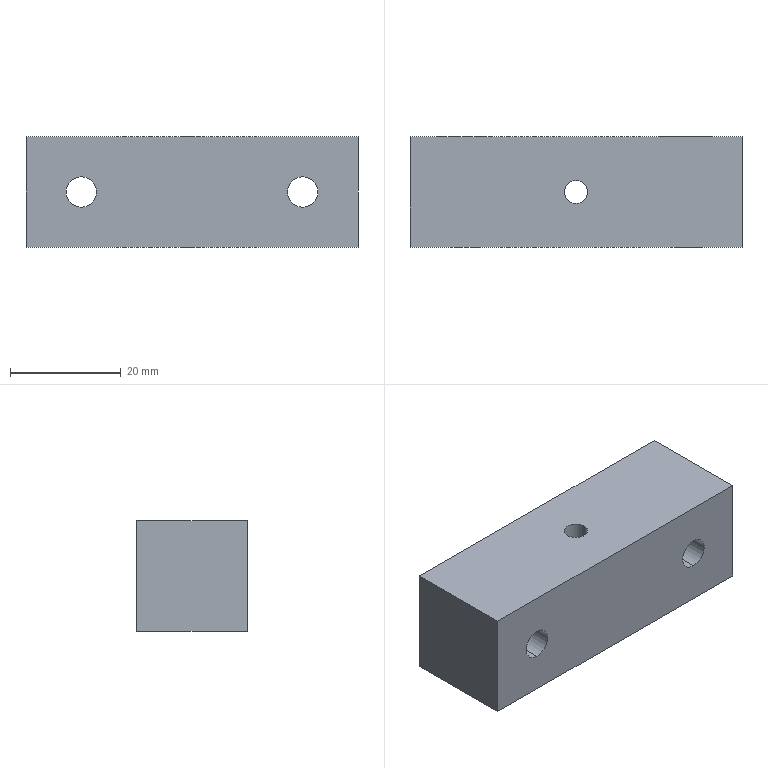Part | SolidWorks | features HoleWzd 2, Extrusion 1 | 1 solid | 18 faces | box 60 x 20 x 20 mm | volume 22148 mm3 | cylinder 10 | plane 8 | commonest cylinder face diameters 5.5 x4 10 x4 4.2 x2
STEP:
#1=CARTESIAN_POINT('',(-2.1,0.,-10.));
#2=VERTEX_POINT('',#1);
#3=CARTESIAN_POINT('',(2.1,0.,-10.));
#4=VERTEX_POINT('',#3);
#5=CARTESIAN_POINT('',(0.,0.,-10.));
#6=DIRECTION('',(0.,0.,1.));
#7=DIRECTION('',(1.,0.,0.));
#8=AXIS2_PLACEMENT_3D('',#5,#6,#7);
#9=CIRCLE('',#8,2.1);
#10=EDGE_CURVE('',#2,#4,#9,.T.);
#11=ORIENTED_EDGE('',*,*,#10,.F.);
#12=CARTESIAN_POINT('',(-2.1,0.,10.));
#13=VERTEX_POINT('',#12);
#14=CARTESIAN_POINT('',(-2.1,0.,10.));
#15=DIRECTION('',(0.,0.,1.));
#16=VECTOR('',#15,1000.);
#17=LINE('',#14,#16);
#18=EDGE_CURVE('',#2,#13,#17,.T.);
#19=ORIENTED_EDGE('',*,*,#18,.T.);
#20=CARTESIAN_POINT('',(2.1,0.,10.));
#21=VERTEX_POINT('',#20);
#22=CARTESIAN_POINT('',(0.,0.,10.));
#23=DIRECTION('',(0.,0.,1.));
#24=DIRECTION('',(1.,0.,0.));
#25=AXIS2_PLACEMENT_3D('',#22,#23,#24);
#26=CIRCLE('',#25,2.1);
#27=EDGE_CURVE('',#13,#21,#26,.T.);
#28=ORIENTED_EDGE('',*,*,#27,.T.);
#29=CARTESIAN_POINT('',(2.1,0.,10.));
#30=DIRECTION('',(0.,0.,1.));
#31=VECTOR('',#30,1000.);
#32=LINE('',#29,#31);
#33=EDGE_CURVE('',#4,#21,#32,.T.);
#34=ORIENTED_EDGE('',*,*,#33,.F.);
#35=EDGE_LOOP('',(#11,#19,#28,#34));
#36=FACE_OUTER_BOUND('',#35,.T.);
#37=CARTESIAN_POINT('',(0.,0.,10.));
#38=DIRECTION('',(0.,0.,1.));
#39=DIRECTION('',(1.,0.,0.));
#40=AXIS2_PLACEMENT_3D('',#37,#38,#39);
#41=CYLINDRICAL_SURFACE('',#40,2.1);
#42=ADVANCED_FACE('',(#36),#41,.F.);
#43=CARTESIAN_POINT('',(20.,4.3,-5.));
#44=VERTEX_POINT('',#43);
#45=CARTESIAN_POINT('',(20.,4.3,5.));
#46=VERTEX_POINT('',#45);
#47=CARTESIAN_POINT('',(20.,4.3,0.));
#48=DIRECTION('',(0.,1.,0.));
#49=DIRECTION('',(0.,0.,1.));
#50=AXIS2_PLACEMENT_3D('',#47,#48,#49);
#51=CIRCLE('',#50,5.);
#52=EDGE_CURVE('',#44,#46,#51,.T.);
#53=ORIENTED_EDGE('',*,*,#52,.F.);
#54=CARTESIAN_POINT('',(20.,10.,-5.));
#55=VERTEX_POINT('',#54);
#56=CARTESIAN_POINT('',(20.,10.,-5.));
#57=DIRECTION('',(0.,1.,0.));
#58=VECTOR('',#57,1000.);
#59=LINE('',#56,#58);
#60=EDGE_CURVE('',#44,#55,#59,.T.);
#61=ORIENTED_EDGE('',*,*,#60,.T.);
#62=CARTESIAN_POINT('',(20.,10.,5.));
#63=VERTEX_POINT('',#62);
#64=CARTESIAN_POINT('',(20.,10.,0.));
#65=DIRECTION('',(0.,1.,0.));
#66=DIRECTION('',(0.,0.,1.));
#67=AXIS2_PLACEMENT_3D('',#64,#65,#66);
#68=CIRCLE('',#67,5.);
#69=EDGE_CURVE('',#55,#63,#68,.T.);
#70=ORIENTED_EDGE('',*,*,#69,.T.);
#71=CARTESIAN_POINT('',(20.,10.,5.));
#72=DIRECTION('',(0.,1.,0.));
#73=VECTOR('',#72,1000.);
#74=LINE('',#71,#73);
#75=EDGE_CURVE('',#46,#63,#74,.T.);
#76=ORIENTED_EDGE('',*,*,#75,.F.);
#77=EDGE_LOOP('',(#53,#61,#70,#76));
#78=FACE_OUTER_BOUND('',#77,.T.);
#79=CARTESIAN_POINT('',(20.,10.,0.));
#80=DIRECTION('',(0.,1.,0.));
#81=DIRECTION('',(0.,0.,1.));
#82=AXIS2_PLACEMENT_3D('',#79,#80,#81);
#83=CYLINDRICAL_SURFACE('',#82,5.);
#84=ADVANCED_FACE('',(#78),#83,.F.);
#85=CARTESIAN_POINT('',(20.,-10.,-2.75));
#86=VERTEX_POINT('',#85);
#87=CARTESIAN_POINT('',(20.,-10.,2.75));
#88=VERTEX_POINT('',#87);
#89=CARTESIAN_POINT('',(20.,-10.,0.));
#90=DIRECTION('',(0.,1.,0.));
#91=DIRECTION('',(0.,0.,1.));
#92=AXIS2_PLACEMENT_3D('',#89,#90,#91);
#93=CIRCLE('',#92,2.75);
#94=EDGE_CURVE('',#86,#88,#93,.T.);
#95=ORIENTED_EDGE('',*,*,#94,.F.);
#96=CARTESIAN_POINT('',(20.,4.3,-2.75));
#97=VERTEX_POINT('',#96);
#98=CARTESIAN_POINT('',(20.,10.,-2.75));
#99=DIRECTION('',(0.,1.,0.));
#100=VECTOR('',#99,1000.);
#101=LINE('',#98,#100);
#102=EDGE_CURVE('',#86,#97,#101,.T.);
#103=ORIENTED_EDGE('',*,*,#102,.T.);
#104=CARTESIAN_POINT('',(20.,4.3,2.75));
#105=VERTEX_POINT('',#104);
#106=CARTESIAN_POINT('',(20.,4.3,0.));
#107=DIRECTION('',(0.,1.,0.));
#108=DIRECTION('',(0.,0.,1.));
#109=AXIS2_PLACEMENT_3D('',#106,#107,#108);
#110=CIRCLE('',#109,2.75);
#111=EDGE_CURVE('',#97,#105,#110,.T.);
#112=ORIENTED_EDGE('',*,*,#111,.T.);
#113=CARTESIAN_POINT('',(20.,10.,2.75));
#114=DIRECTION('',(0.,1.,0.));
#115=VECTOR('',#114,1000.);
#116=LINE('',#113,#115);
#117=EDGE_CURVE('',#88,#105,#116,.T.);
#118=ORIENTED_EDGE('',*,*,#117,.F.);
#119=EDGE_LOOP('',(#95,#103,#112,#118));
#120=FACE_OUTER_BOUND('',#119,.T.);
#121=CARTESIAN_POINT('',(20.,10.,0.));
#122=DIRECTION('',(0.,1.,0.));
#123=DIRECTION('',(0.,0.,1.));
#124=AXIS2_PLACEMENT_3D('',#121,#122,#123);
#125=CYLINDRICAL_SURFACE('',#124,2.75);
#126=ADVANCED_FACE('',(#120),#125,.F.);
#127=CARTESIAN_POINT('',(-20.,4.3,-5.));
#128=VERTEX_POINT('',#127);
#129=CARTESIAN_POINT('',(-20.,4.3,5.));
#130=VERTEX_POINT('',#129);
#131=CARTESIAN_POINT('',(-20.,4.3,0.));
#132=DIRECTION('',(0.,1.,0.));
#133=DIRECTION('',(0.,0.,1.));
#134=AXIS2_PLACEMENT_3D('',#131,#132,#133);
#135=CIRCLE('',#134,5.);
#136=EDGE_CURVE('',#128,#130,#135,.T.);
#137=ORIENTED_EDGE('',*,*,#136,.F.);
#138=CARTESIAN_POINT('',(-20.,10.,-5.));
#139=VERTEX_POINT('',#138);
#140=CARTESIAN_POINT('',(-20.,10.,-5.));
#141=DIRECTION('',(0.,1.,0.));
#142=VECTOR('',#141,1000.);
#143=LINE('',#140,#142);
#144=EDGE_CURVE('',#128,#139,#143,.T.);
#145=ORIENTED_EDGE('',*,*,#144,.T.);
#146=CARTESIAN_POINT('',(-20.,10.,5.));
#147=VERTEX_POINT('',#146);
#148=CARTESIAN_POINT('',(-20.,10.,0.));
#149=DIRECTION('',(0.,1.,0.));
#150=DIRECTION('',(0.,0.,1.));
#151=AXIS2_PLACEMENT_3D('',#148,#149,#150);
#152=CIRCLE('',#151,5.);
#153=EDGE_CURVE('',#139,#147,#152,.T.);
#154=ORIENTED_EDGE('',*,*,#153,.T.);
#155=CARTESIAN_POINT('',(-20.,10.,5.));
#156=DIRECTION('',(0.,1.,0.));
#157=VECTOR('',#156,1000.);
#158=LINE('',#155,#157);
#159=EDGE_CURVE('',#130,#147,#158,.T.);
#160=ORIENTED_EDGE('',*,*,#159,.F.);
#161=EDGE_LOOP('',(#137,#145,#154,#160));
#162=FACE_OUTER_BOUND('',#161,.T.);
#163=CARTESIAN_POINT('',(-20.,10.,0.));
#164=DIRECTION('',(0.,1.,0.));
#165=DIRECTION('',(0.,0.,1.));
#166=AXIS2_PLACEMENT_3D('',#163,#164,#165);
#167=CYLINDRICAL_SURFACE('',#166,5.);
#168=ADVANCED_FACE('',(#162),#167,.F.);
#169=CARTESIAN_POINT('',(-20.,-10.,-2.75));
#170=VERTEX_POINT('',#169);
#171=CARTESIAN_POINT('',(-20.,-10.,2.75));
#172=VERTEX_POINT('',#171);
#173=CARTESIAN_POINT('',(-20.,-10.,0.));
#174=DIRECTION('',(0.,1.,0.));
#175=DIRECTION('',(0.,0.,1.));
#176=AXIS2_PLACEMENT_3D('',#173,#174,#175);
#177=CIRCLE('',#176,2.75);
#178=EDGE_CURVE('',#170,#172,#177,.T.);
#179=ORIENTED_EDGE('',*,*,#178,.F.);
#180=CARTESIAN_POINT('',(-20.,4.3,-2.75));
#181=VERTEX_POINT('',#180);
#182=CARTESIAN_POINT('',(-20.,10.,-2.75));
#183=DIRECTION('',(0.,1.,0.));
#184=VECTOR('',#183,1000.);
#185=LINE('',#182,#184);
#186=EDGE_CURVE('',#170,#181,#185,.T.);
#187=ORIENTED_EDGE('',*,*,#186,.T.);
#188=CARTESIAN_POINT('',(-20.,4.3,2.75));
#189=VERTEX_POINT('',#188);
#190=CARTESIAN_POINT('',(-20.,4.3,0.));
#191=DIRECTION('',(0.,1.,0.));
#192=DIRECTION('',(0.,0.,1.));
#193=AXIS2_PLACEMENT_3D('',#190,#191,#192);
#194=CIRCLE('',#193,2.75);
#195=EDGE_CURVE('',#181,#189,#194,.T.);
#196=ORIENTED_EDGE('',*,*,#195,.T.);
#197=CARTESIAN_POINT('',(-20.,10.,2.75));
#198=DIRECTION('',(0.,1.,0.));
#199=VECTOR('',#198,1000.);
#200=LINE('',#197,#199);
#201=EDGE_CURVE('',#172,#189,#200,.T.);
#202=ORIENTED_EDGE('',*,*,#201,.F.);
#203=EDGE_LOOP('',(#179,#187,#196,#202));
#204=FACE_OUTER_BOUND('',#203,.T.);
#205=CARTESIAN_POINT('',(-20.,10.,0.));
#206=DIRECTION('',(0.,1.,0.));
#207=DIRECTION('',(0.,0.,1.));
#208=AXIS2_PLACEMENT_3D('',#205,#206,#207);
#209=CYLINDRICAL_SURFACE('',#208,2.75);
#210=ADVANCED_FACE('',(#204),#209,.F.);
#211=CARTESIAN_POINT('',(30.,-10.,10.));
#212=VERTEX_POINT('',#211);
#213=CARTESIAN_POINT('',(30.,-10.,-10.));
#214=VERTEX_POINT('',#213);
#215=CARTESIAN_POINT('',(30.,-10.,10.));
#216=DIRECTION('',(0.,0.,-1.));
#217=VECTOR('',#216,1000.);
#218=LINE('',#215,#217);
#219=EDGE_CURVE('',#212,#214,#218,.T.);
#220=ORIENTED_EDGE('',*,*,#219,.T.);
#221=CARTESIAN_POINT('',(30.,10.,-10.));
#222=VERTEX_POINT('',#221);
#223=CARTESIAN_POINT('',(30.,10.,-10.));
#224=DIRECTION('',(0.,-1.,0.));
#225=VECTOR('',#224,1000.);
#226=LINE('',#223,#225);
#227=EDGE_CURVE('',#222,#214,#226,.T.);
#228=ORIENTED_EDGE('',*,*,#227,.F.);
#229=CARTESIAN_POINT('',(30.,10.,10.));
#230=VERTEX_POINT('',#229);
#231=CARTESIAN_POINT('',(30.,10.,10.));
#232=DIRECTION('',(0.,0.,-1.));
#233=VECTOR('',#232,1000.);
#234=LINE('',#231,#233);
#235=EDGE_CURVE('',#230,#222,#234,.T.);
#236=ORIENTED_EDGE('',*,*,#235,.F.);
#237=CARTESIAN_POINT('',(30.,10.,10.));
#238=DIRECTION('',(0.,-1.,0.));
#239=VECTOR('',#238,1000.);
#240=LINE('',#237,#239);
#241=EDGE_CURVE('',#230,#212,#240,.T.);
#242=ORIENTED_EDGE('',*,*,#241,.T.);
#243=EDGE_LOOP('',(#220,#228,#236,#242));
#244=FACE_OUTER_BOUND('',#243,.T.);
#245=CARTESIAN_POINT('',(30.,10.,10.));
#246=DIRECTION('',(-1.,0.,0.));
#247=DIRECTION('',(0.,0.,1.));
#248=AXIS2_PLACEMENT_3D('',#245,#246,#247);
#249=PLANE('',#248);
#250=ADVANCED_FACE('',(#244),#249,.F.);
#251=CARTESIAN_POINT('',(0.,0.,-10.));
#252=DIRECTION('',(0.,0.,1.));
#253=DIRECTION('',(1.,0.,0.));
#254=AXIS2_PLACEMENT_3D('',#251,#252,#253);
#255=CIRCLE('',#254,2.1);
#256=EDGE_CURVE('',#4,#2,#255,.T.);
#257=ORIENTED_EDGE('',*,*,#256,.T.);
#258=ORIENTED_EDGE('',*,*,#10,.T.);
#259=EDGE_LOOP('',(#257,#258));
#260=FACE_BOUND('',#259,.T.);
#261=CARTESIAN_POINT('',(-30.,-10.,-10.));
#262=VERTEX_POINT('',#261);
#263=CARTESIAN_POINT('',(-30.,-10.,-10.));
#264=DIRECTION('',(-1.,0.,0.));
#265=VECTOR('',#264,1000.);
#266=LINE('',#263,#265);
#267=EDGE_CURVE('',#214,#262,#266,.T.);
#268=ORIENTED_EDGE('',*,*,#267,.T.);
#269=CARTESIAN_POINT('',(-30.,10.,-10.));
#270=VERTEX_POINT('',#269);
#271=CARTESIAN_POINT('',(-30.,10.,-10.));
#272=DIRECTION('',(0.,-1.,0.));
#273=VECTOR('',#272,1000.);
#274=LINE('',#271,#273);
#275=EDGE_CURVE('',#270,#262,#274,.T.);
#276=ORIENTED_EDGE('',*,*,#275,.F.);
#277=CARTESIAN_POINT('',(-30.,10.,-10.));
#278=DIRECTION('',(-1.,0.,0.));
#279=VECTOR('',#278,1000.);
#280=LINE('',#277,#279);
#281=EDGE_CURVE('',#222,#270,#280,.T.);
#282=ORIENTED_EDGE('',*,*,#281,.F.);
#283=ORIENTED_EDGE('',*,*,#227,.T.);
#284=EDGE_LOOP('',(#268,#276,#282,#283));
#285=FACE_OUTER_BOUND('',#284,.T.);
#286=CARTESIAN_POINT('',(-30.,10.,-10.));
#287=DIRECTION('',(0.,0.,1.));
#288=DIRECTION('',(1.,0.,0.));
#289=AXIS2_PLACEMENT_3D('',#286,#287,#288);
#290=PLANE('',#289);
#291=ADVANCED_FACE('',(#260,#285),#290,.F.);
#292=CARTESIAN_POINT('',(-30.,-10.,10.));
#293=VERTEX_POINT('',#292);
#294=CARTESIAN_POINT('',(-30.,-10.,10.));
#295=DIRECTION('',(0.,0.,1.));
#296=VECTOR('',#295,1000.);
#297=LINE('',#294,#296);
#298=EDGE_CURVE('',#262,#293,#297,.T.);
#299=ORIENTED_EDGE('',*,*,#298,.T.);
#300=CARTESIAN_POINT('',(-30.,10.,10.));
#301=VERTEX_POINT('',#300);
#302=CARTESIAN_POINT('',(-30.,10.,10.));
#303=DIRECTION('',(0.,-1.,0.));
#304=VECTOR('',#303,1000.);
#305=LINE('',#302,#304);
#306=EDGE_CURVE('',#301,#293,#305,.T.);
#307=ORIENTED_EDGE('',*,*,#306,.F.);
#308=CARTESIAN_POINT('',(-30.,10.,10.));
#309=DIRECTION('',(0.,0.,1.));
#310=VECTOR('',#309,1000.);
#311=LINE('',#308,#310);
#312=EDGE_CURVE('',#270,#301,#311,.T.);
#313=ORIENTED_EDGE('',*,*,#312,.F.);
#314=ORIENTED_EDGE('',*,*,#275,.T.);
#315=EDGE_LOOP('',(#299,#307,#313,#314));
#316=FACE_OUTER_BOUND('',#315,.T.);
#317=CARTESIAN_POINT('',(-30.,10.,10.));
#318=DIRECTION('',(1.,0.,0.));
#319=DIRECTION('',(0.,0.,-1.));
#320=AXIS2_PLACEMENT_3D('',#317,#318,#319);
#321=PLANE('',#320);
#322=ADVANCED_FACE('',(#316),#321,.F.);
#323=CARTESIAN_POINT('',(0.,0.,10.));
#324=DIRECTION('',(0.,0.,1.));
#325=DIRECTION('',(1.,0.,0.));
#326=AXIS2_PLACEMENT_3D('',#323,#324,#325);
#327=CIRCLE('',#326,2.1);
#328=EDGE_CURVE('',#21,#13,#327,.T.);
#329=ORIENTED_EDGE('',*,*,#328,.F.);
#330=ORIENTED_EDGE('',*,*,#27,.F.);
#331=EDGE_LOOP('',(#329,#330));
#332=FACE_BOUND('',#331,.T.);
#333=CARTESIAN_POINT('',(-30.,-10.,10.));
#334=DIRECTION('',(1.,0.,0.));
#335=VECTOR('',#334,1000.);
#336=LINE('',#333,#335);
#337=EDGE_CURVE('',#293,#212,#336,.T.);
#338=ORIENTED_EDGE('',*,*,#337,.T.);
#339=ORIENTED_EDGE('',*,*,#241,.F.);
#340=CARTESIAN_POINT('',(-30.,10.,10.));
#341=DIRECTION('',(1.,0.,0.));
#342=VECTOR('',#341,1000.);
#343=LINE('',#340,#342);
#344=EDGE_CURVE('',#301,#230,#343,.T.);
#345=ORIENTED_EDGE('',*,*,#344,.F.);
#346=ORIENTED_EDGE('',*,*,#306,.T.);
#347=EDGE_LOOP('',(#338,#339,#345,#346));
#348=FACE_OUTER_BOUND('',#347,.T.);
#349=CARTESIAN_POINT('',(-30.,10.,10.));
#350=DIRECTION('',(0.,0.,-1.));
#351=DIRECTION('',(-1.,0.,0.));
#352=AXIS2_PLACEMENT_3D('',#349,#350,#351);
#353=PLANE('',#352);
#354=ADVANCED_FACE('',(#332,#348),#353,.F.);
#355=CARTESIAN_POINT('',(20.,10.,0.));
#356=DIRECTION('',(0.,1.,0.));
#357=DIRECTION('',(0.,0.,1.));
#358=AXIS2_PLACEMENT_3D('',#355,#356,#357);
#359=CIRCLE('',#358,5.);
#360=EDGE_CURVE('',#63,#55,#359,.T.);
#361=ORIENTED_EDGE('',*,*,#360,.F.);
#362=ORIENTED_EDGE('',*,*,#69,.F.);
#363=EDGE_LOOP('',(#361,#362));
#364=FACE_BOUND('',#363,.T.);
#365=CARTESIAN_POINT('',(-20.,10.,0.));
#366=DIRECTION('',(0.,1.,0.));
#367=DIRECTION('',(0.,0.,1.));
#368=AXIS2_PLACEMENT_3D('',#365,#366,#367);
#369=CIRCLE('',#368,5.);
#370=EDGE_CURVE('',#147,#139,#369,.T.);
#371=ORIENTED_EDGE('',*,*,#370,.F.);
#372=ORIENTED_EDGE('',*,*,#153,.F.);
#373=EDGE_LOOP('',(#371,#372));
#374=FACE_BOUND('',#373,.T.);
#375=ORIENTED_EDGE('',*,*,#235,.T.);
#376=ORIENTED_EDGE('',*,*,#281,.T.);
#377=ORIENTED_EDGE('',*,*,#312,.T.);
#378=ORIENTED_EDGE('',*,*,#344,.T.);
#379=EDGE_LOOP('',(#375,#376,#377,#378));
#380=FACE_OUTER_BOUND('',#379,.T.);
#381=CARTESIAN_POINT('',(0.,10.,0.));
#382=DIRECTION('',(0.,-1.,0.));
#383=DIRECTION('',(0.,0.,-1.));
#384=AXIS2_PLACEMENT_3D('',#381,#382,#383);
#385=PLANE('',#384);
#386=ADVANCED_FACE('',(#364,#374,#380),#385,.F.);
#387=CARTESIAN_POINT('',(20.,-10.,0.));
#388=DIRECTION('',(0.,1.,0.));
#389=DIRECTION('',(0.,0.,1.));
#390=AXIS2_PLACEMENT_3D('',#387,#388,#389);
#391=CIRCLE('',#390,2.75);
#392=EDGE_CURVE('',#88,#86,#391,.T.);
#393=ORIENTED_EDGE('',*,*,#392,.T.);
#394=ORIENTED_EDGE('',*,*,#94,.T.);
#395=EDGE_LOOP('',(#393,#394));
#396=FACE_BOUND('',#395,.T.);
#397=CARTESIAN_POINT('',(-20.,-10.,0.));
#398=DIRECTION('',(0.,1.,0.));
#399=DIRECTION('',(0.,0.,1.));
#400=AXIS2_PLACEMENT_3D('',#397,#398,#399);
#401=CIRCLE('',#400,2.75);
#402=EDGE_CURVE('',#172,#170,#401,.T.);
#403=ORIENTED_EDGE('',*,*,#402,.T.);
#404=ORIENTED_EDGE('',*,*,#178,.T.);
#405=EDGE_LOOP('',(#403,#404));
#406=FACE_BOUND('',#405,.T.);
#407=ORIENTED_EDGE('',*,*,#219,.F.);
#408=ORIENTED_EDGE('',*,*,#337,.F.);
#409=ORIENTED_EDGE('',*,*,#298,.F.);
#410=ORIENTED_EDGE('',*,*,#267,.F.);
#411=EDGE_LOOP('',(#407,#408,#409,#410));
#412=FACE_OUTER_BOUND('',#411,.T.);
#413=CARTESIAN_POINT('',(0.,-10.,0.));
#414=DIRECTION('',(0.,-1.,0.));
#415=DIRECTION('',(0.,0.,-1.));
#416=AXIS2_PLACEMENT_3D('',#413,#414,#415);
#417=PLANE('',#416);
#418=ADVANCED_FACE('',(#396,#406,#412),#417,.T.);
#419=ORIENTED_EDGE('',*,*,#186,.F.);
#420=ORIENTED_EDGE('',*,*,#402,.F.);
#421=ORIENTED_EDGE('',*,*,#201,.T.);
#422=CARTESIAN_POINT('',(-20.,4.3,0.));
#423=DIRECTION('',(0.,1.,0.));
#424=DIRECTION('',(0.,0.,1.));
#425=AXIS2_PLACEMENT_3D('',#422,#423,#424);
#426=CIRCLE('',#425,2.75);
#427=EDGE_CURVE('',#189,#181,#426,.T.);
#428=ORIENTED_EDGE('',*,*,#427,.T.);
#429=EDGE_LOOP('',(#419,#420,#421,#428));
#430=FACE_OUTER_BOUND('',#429,.T.);
#431=CARTESIAN_POINT('',(-20.,10.,0.));
#432=DIRECTION('',(0.,1.,0.));
#433=DIRECTION('',(0.,0.,1.));
#434=AXIS2_PLACEMENT_3D('',#431,#432,#433);
#435=CYLINDRICAL_SURFACE('',#434,2.75);
#436=ADVANCED_FACE('',(#430),#435,.F.);
#437=ORIENTED_EDGE('',*,*,#427,.F.);
#438=ORIENTED_EDGE('',*,*,#195,.F.);
#439=EDGE_LOOP('',(#437,#438));
#440=FACE_BOUND('',#439,.T.);
#441=CARTESIAN_POINT('',(-20.,4.3,0.));
#442=DIRECTION('',(0.,1.,0.));
#443=DIRECTION('',(0.,0.,1.));
#444=AXIS2_PLACEMENT_3D('',#441,#442,#443);
#445=CIRCLE('',#444,5.);
#446=EDGE_CURVE('',#130,#128,#445,.T.);
#447=ORIENTED_EDGE('',*,*,#446,.T.);
#448=ORIENTED_EDGE('',*,*,#136,.T.);
#449=EDGE_LOOP('',(#447,#448));
#450=FACE_OUTER_BOUND('',#449,.T.);
#451=CARTESIAN_POINT('',(-17.25,4.3,0.));
#452=DIRECTION('',(0.,-1.,0.));
#453=DIRECTION('',(0.,0.,-1.));
#454=AXIS2_PLACEMENT_3D('',#451,#452,#453);
#455=PLANE('',#454);
#456=ADVANCED_FACE('',(#440,#450),#455,.F.);
#457=ORIENTED_EDGE('',*,*,#144,.F.);
#458=ORIENTED_EDGE('',*,*,#446,.F.);
#459=ORIENTED_EDGE('',*,*,#159,.T.);
#460=ORIENTED_EDGE('',*,*,#370,.T.);
#461=EDGE_LOOP('',(#457,#458,#459,#460));
#462=FACE_OUTER_BOUND('',#461,.T.);
#463=CARTESIAN_POINT('',(-20.,10.,0.));
#464=DIRECTION('',(0.,1.,0.));
#465=DIRECTION('',(0.,0.,1.));
#466=AXIS2_PLACEMENT_3D('',#463,#464,#465);
#467=CYLINDRICAL_SURFACE('',#466,5.);
#468=ADVANCED_FACE('',(#462),#467,.F.);
#469=ORIENTED_EDGE('',*,*,#102,.F.);
#470=ORIENTED_EDGE('',*,*,#392,.F.);
#471=ORIENTED_EDGE('',*,*,#117,.T.);
#472=CARTESIAN_POINT('',(20.,4.3,0.));
#473=DIRECTION('',(0.,1.,0.));
#474=DIRECTION('',(0.,0.,1.));
#475=AXIS2_PLACEMENT_3D('',#472,#473,#474);
#476=CIRCLE('',#475,2.75);
#477=EDGE_CURVE('',#105,#97,#476,.T.);
#478=ORIENTED_EDGE('',*,*,#477,.T.);
#479=EDGE_LOOP('',(#469,#470,#471,#478));
#480=FACE_OUTER_BOUND('',#479,.T.);
#481=CARTESIAN_POINT('',(20.,10.,0.));
#482=DIRECTION('',(0.,1.,0.));
#483=DIRECTION('',(0.,0.,1.));
#484=AXIS2_PLACEMENT_3D('',#481,#482,#483);
#485=CYLINDRICAL_SURFACE('',#484,2.75);
#486=ADVANCED_FACE('',(#480),#485,.F.);
#487=ORIENTED_EDGE('',*,*,#477,.F.);
#488=ORIENTED_EDGE('',*,*,#111,.F.);
#489=EDGE_LOOP('',(#487,#488));
#490=FACE_BOUND('',#489,.T.);
#491=CARTESIAN_POINT('',(20.,4.3,0.));
#492=DIRECTION('',(0.,1.,0.));
#493=DIRECTION('',(0.,0.,1.));
#494=AXIS2_PLACEMENT_3D('',#491,#492,#493);
#495=CIRCLE('',#494,5.);
#496=EDGE_CURVE('',#46,#44,#495,.T.);
#497=ORIENTED_EDGE('',*,*,#496,.T.);
#498=ORIENTED_EDGE('',*,*,#52,.T.);
#499=EDGE_LOOP('',(#497,#498));
#500=FACE_OUTER_BOUND('',#499,.T.);
#501=CARTESIAN_POINT('',(22.75,4.3,0.));
#502=DIRECTION('',(0.,-1.,0.));
#503=DIRECTION('',(0.,0.,-1.));
#504=AXIS2_PLACEMENT_3D('',#501,#502,#503);
#505=PLANE('',#504);
#506=ADVANCED_FACE('',(#490,#500),#505,.F.);
#507=ORIENTED_EDGE('',*,*,#60,.F.);
#508=ORIENTED_EDGE('',*,*,#496,.F.);
#509=ORIENTED_EDGE('',*,*,#75,.T.);
#510=ORIENTED_EDGE('',*,*,#360,.T.);
#511=EDGE_LOOP('',(#507,#508,#509,#510));
#512=FACE_OUTER_BOUND('',#511,.T.);
#513=CARTESIAN_POINT('',(20.,10.,0.));
#514=DIRECTION('',(0.,1.,0.));
#515=DIRECTION('',(0.,0.,1.));
#516=AXIS2_PLACEMENT_3D('',#513,#514,#515);
#517=CYLINDRICAL_SURFACE('',#516,5.);
#518=ADVANCED_FACE('',(#512),#517,.F.);
#519=ORIENTED_EDGE('',*,*,#18,.F.);
#520=ORIENTED_EDGE('',*,*,#256,.F.);
#521=ORIENTED_EDGE('',*,*,#33,.T.);
#522=ORIENTED_EDGE('',*,*,#328,.T.);
#523=EDGE_LOOP('',(#519,#520,#521,#522));
#524=FACE_OUTER_BOUND('',#523,.T.);
#525=CARTESIAN_POINT('',(0.,0.,10.));
#526=DIRECTION('',(0.,0.,1.));
#527=DIRECTION('',(1.,0.,0.));
#528=AXIS2_PLACEMENT_3D('',#525,#526,#527);
#529=CYLINDRICAL_SURFACE('',#528,2.1);
#530=ADVANCED_FACE('',(#524),#529,.F.);
#531=CLOSED_SHELL('',(#42,#84,#126,#168,#210,#250,#291,#322,#354,#386,#418,#436,#456,#468,#486,#506,#518,#530));
#532=MANIFOLD_SOLID_BREP('',#531);
#533=CARTESIAN_POINT('',(0.,0.,0.));
#534=DIRECTION('',(0.,0.,1.));
#535=DIRECTION('',(1.,0.,0.));
#536=AXIS2_PLACEMENT_3D('',#533,#534,#535);
#537=(LENGTH_UNIT()NAMED_UNIT(*)SI_UNIT(.MILLI.,.METRE.));
#538=UNCERTAINTY_MEASURE_WITH_UNIT(LENGTH_MEASURE(0.00001),#537,'','');
#539=(NAMED_UNIT(*)PLANE_ANGLE_UNIT()SI_UNIT($,.RADIAN.));
#540=(NAMED_UNIT(*)SI_UNIT($,.STERADIAN.)SOLID_ANGLE_UNIT());
#541=(GEOMETRIC_REPRESENTATION_CONTEXT(3)GLOBAL_UNCERTAINTY_ASSIGNED_CONTEXT((#538))GLOBAL_UNIT_ASSIGNED_CONTEXT((#537,#539,#540))REPRESENTATION_CONTEXT('',''));
#542=ADVANCED_BREP_SHAPE_REPRESENTATION('',(#532,#536),#541);